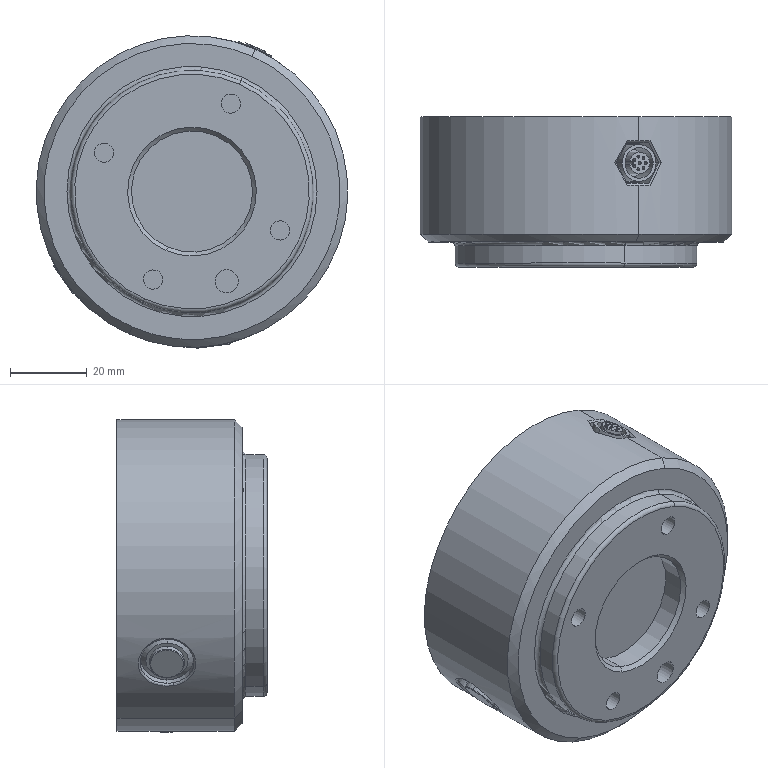Part | SolidWorks | features BaseBody 2 | 2 solids | 115 faces | box 81 x 39 x 81.209 mm | volume 180493 mm3 | cylinder 47 | plane 41 | cone 11 | torus 8 | spline 8 | commonest cylinder face diameters 0.8 x17 5 x8 9 x4 14 x4 5.6 x2 6 x2